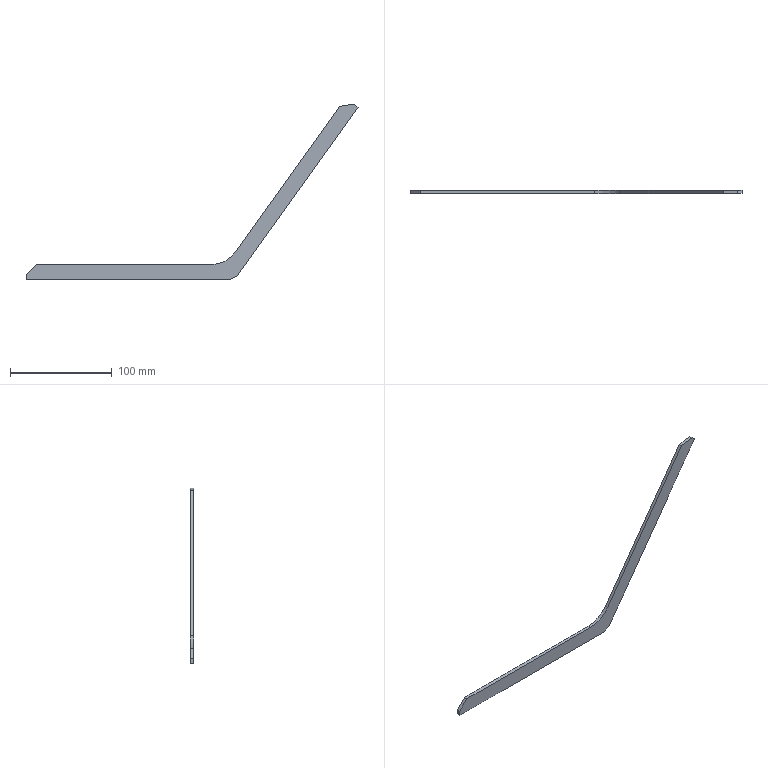Part | SolidWorks | features FlatPattern 1, SMBaseFlange 1, SheetMetal 1 | 1 solid | 12 faces | box 326.5 x 3.2 x 172.806 mm | volume 19256 mm3 | plane 11 | cylinder 1 | commonest cylinder face diameters 60 x1
STEP:
#1=CARTESIAN_POINT('',(0.,0.,0.));
#2=VERTEX_POINT('',#1);
#3=CARTESIAN_POINT('',(0.,0.,5.));
#4=VERTEX_POINT('',#3);
#5=CARTESIAN_POINT('',(0.,0.,0.));
#6=DIRECTION('',(0.,0.,1.));
#7=VECTOR('',#6,1000.);
#8=LINE('',#5,#7);
#9=EDGE_CURVE('',#2,#4,#8,.T.);
#10=ORIENTED_EDGE('',*,*,#9,.F.);
#11=CARTESIAN_POINT('',(0.,-3.2,0.));
#12=VERTEX_POINT('',#11);
#13=CARTESIAN_POINT('',(0.,-3.2,0.));
#14=DIRECTION('',(0.,1.,0.));
#15=VECTOR('',#14,1000.);
#16=LINE('',#13,#15);
#17=EDGE_CURVE('',#12,#2,#16,.T.);
#18=ORIENTED_EDGE('',*,*,#17,.F.);
#19=CARTESIAN_POINT('',(0.,-3.2,5.));
#20=VERTEX_POINT('',#19);
#21=CARTESIAN_POINT('',(0.,-3.2,0.));
#22=DIRECTION('',(0.,0.,1.));
#23=VECTOR('',#22,1000.);
#24=LINE('',#21,#23);
#25=EDGE_CURVE('',#12,#20,#24,.T.);
#26=ORIENTED_EDGE('',*,*,#25,.T.);
#27=CARTESIAN_POINT('',(0.,-3.2,5.));
#28=DIRECTION('',(0.,1.,0.));
#29=VECTOR('',#28,1000.);
#30=LINE('',#27,#29);
#31=EDGE_CURVE('',#20,#4,#30,.T.);
#32=ORIENTED_EDGE('',*,*,#31,.T.);
#33=EDGE_LOOP('',(#10,#18,#26,#32));
#34=FACE_OUTER_BOUND('',#33,.T.);
#35=CARTESIAN_POINT('',(0.,-3.2,0.));
#36=DIRECTION('',(-1.,0.,0.));
#37=DIRECTION('',(0.,0.,1.));
#38=AXIS2_PLACEMENT_3D('',#35,#36,#37);
#39=PLANE('',#38);
#40=ADVANCED_FACE('',(#34),#39,.T.);
#41=CARTESIAN_POINT('',(200.,0.,0.));
#42=VERTEX_POINT('',#41);
#43=CARTESIAN_POINT('',(0.,0.,0.));
#44=DIRECTION('',(-1.,0.,0.));
#45=VECTOR('',#44,1000.);
#46=LINE('',#43,#45);
#47=EDGE_CURVE('',#42,#2,#46,.T.);
#48=ORIENTED_EDGE('',*,*,#47,.F.);
#49=CARTESIAN_POINT('',(200.,-3.2,0.));
#50=VERTEX_POINT('',#49);
#51=CARTESIAN_POINT('',(200.,-3.2,0.));
#52=DIRECTION('',(0.,1.,0.));
#53=VECTOR('',#52,1000.);
#54=LINE('',#51,#53);
#55=EDGE_CURVE('',#50,#42,#54,.T.);
#56=ORIENTED_EDGE('',*,*,#55,.F.);
#57=CARTESIAN_POINT('',(0.,-3.2,0.));
#58=DIRECTION('',(-1.,0.,0.));
#59=VECTOR('',#58,1000.);
#60=LINE('',#57,#59);
#61=EDGE_CURVE('',#50,#12,#60,.T.);
#62=ORIENTED_EDGE('',*,*,#61,.T.);
#63=ORIENTED_EDGE('',*,*,#17,.T.);
#64=EDGE_LOOP('',(#48,#56,#62,#63));
#65=FACE_OUTER_BOUND('',#64,.T.);
#66=CARTESIAN_POINT('',(0.,-3.2,0.));
#67=DIRECTION('',(0.,0.,-1.));
#68=DIRECTION('',(-1.,0.,0.));
#69=AXIS2_PLACEMENT_3D('',#66,#67,#68);
#70=PLANE('',#69);
#71=ADVANCED_FACE('',(#65),#70,.T.);
#72=CARTESIAN_POINT('',(207.908,0.,4.067));
#73=VERTEX_POINT('',#72);
#74=CARTESIAN_POINT('',(200.,0.,0.));
#75=DIRECTION('',(-0.8893,0.,-0.4573));
#76=VECTOR('',#75,1000.);
#77=LINE('',#74,#76);
#78=EDGE_CURVE('',#73,#42,#77,.T.);
#79=ORIENTED_EDGE('',*,*,#78,.F.);
#80=CARTESIAN_POINT('',(207.908,-3.2,4.067));
#81=VERTEX_POINT('',#80);
#82=CARTESIAN_POINT('',(207.908,-3.2,4.067));
#83=DIRECTION('',(0.,1.,0.));
#84=VECTOR('',#83,1000.);
#85=LINE('',#82,#84);
#86=EDGE_CURVE('',#81,#73,#85,.T.);
#87=ORIENTED_EDGE('',*,*,#86,.F.);
#88=CARTESIAN_POINT('',(200.,-3.2,0.));
#89=DIRECTION('',(-0.8893,0.,-0.4573));
#90=VECTOR('',#89,1000.);
#91=LINE('',#88,#90);
#92=EDGE_CURVE('',#81,#50,#91,.T.);
#93=ORIENTED_EDGE('',*,*,#92,.T.);
#94=ORIENTED_EDGE('',*,*,#55,.T.);
#95=EDGE_LOOP('',(#79,#87,#93,#94));
#96=FACE_OUTER_BOUND('',#95,.T.);
#97=CARTESIAN_POINT('',(200.,-3.2,0.));
#98=DIRECTION('',(0.4573,0.,-0.8893));
#99=DIRECTION('',(-0.8893,0.,-0.4573));
#100=AXIS2_PLACEMENT_3D('',#97,#98,#99);
#101=PLANE('',#100);
#102=ADVANCED_FACE('',(#96),#101,.T.);
#103=CARTESIAN_POINT('',(326.5,0.,169.897));
#104=VERTEX_POINT('',#103);
#105=CARTESIAN_POINT('',(207.908,0.,4.067));
#106=DIRECTION('',(-0.5817,0.,-0.8134));
#107=VECTOR('',#106,1000.);
#108=LINE('',#105,#107);
#109=EDGE_CURVE('',#104,#73,#108,.T.);
#110=ORIENTED_EDGE('',*,*,#109,.F.);
#111=CARTESIAN_POINT('',(326.5,-3.2,169.897));
#112=VERTEX_POINT('',#111);
#113=CARTESIAN_POINT('',(326.5,-3.2,169.897));
#114=DIRECTION('',(0.,1.,0.));
#115=VECTOR('',#114,1000.);
#116=LINE('',#113,#115);
#117=EDGE_CURVE('',#112,#104,#116,.T.);
#118=ORIENTED_EDGE('',*,*,#117,.F.);
#119=CARTESIAN_POINT('',(207.908,-3.2,4.067));
#120=DIRECTION('',(-0.5817,0.,-0.8134));
#121=VECTOR('',#120,1000.);
#122=LINE('',#119,#121);
#123=EDGE_CURVE('',#112,#81,#122,.T.);
#124=ORIENTED_EDGE('',*,*,#123,.T.);
#125=ORIENTED_EDGE('',*,*,#86,.T.);
#126=EDGE_LOOP('',(#110,#118,#124,#125));
#127=FACE_OUTER_BOUND('',#126,.T.);
#128=CARTESIAN_POINT('',(207.908,-3.2,4.067));
#129=DIRECTION('',(0.8134,0.,-0.5817));
#130=DIRECTION('',(-0.5817,0.,-0.8134));
#131=AXIS2_PLACEMENT_3D('',#128,#129,#130);
#132=PLANE('',#131);
#133=ADVANCED_FACE('',(#127),#132,.T.);
#134=CARTESIAN_POINT('',(322.433,0.,172.806));
#135=VERTEX_POINT('',#134);
#136=CARTESIAN_POINT('',(322.433,0.,172.806));
#137=DIRECTION('',(0.8134,0.,-0.5817));
#138=VECTOR('',#137,1000.);
#139=LINE('',#136,#138);
#140=EDGE_CURVE('',#135,#104,#139,.T.);
#141=ORIENTED_EDGE('',*,*,#140,.F.);
#142=CARTESIAN_POINT('',(322.433,-3.2,172.806));
#143=VERTEX_POINT('',#142);
#144=CARTESIAN_POINT('',(322.433,-3.2,172.806));
#145=DIRECTION('',(0.,1.,0.));
#146=VECTOR('',#145,1000.);
#147=LINE('',#144,#146);
#148=EDGE_CURVE('',#143,#135,#147,.T.);
#149=ORIENTED_EDGE('',*,*,#148,.F.);
#150=CARTESIAN_POINT('',(322.433,-3.2,172.806));
#151=DIRECTION('',(0.8134,0.,-0.5817));
#152=VECTOR('',#151,1000.);
#153=LINE('',#150,#152);
#154=EDGE_CURVE('',#143,#112,#153,.T.);
#155=ORIENTED_EDGE('',*,*,#154,.T.);
#156=ORIENTED_EDGE('',*,*,#117,.T.);
#157=EDGE_LOOP('',(#141,#149,#155,#156));
#158=FACE_OUTER_BOUND('',#157,.T.);
#159=CARTESIAN_POINT('',(322.433,-3.2,172.806));
#160=DIRECTION('',(0.5817,0.,0.8134));
#161=DIRECTION('',(0.8134,0.,-0.5817));
#162=AXIS2_PLACEMENT_3D('',#159,#160,#161);
#163=PLANE('',#162);
#164=ADVANCED_FACE('',(#158),#163,.T.);
#165=CARTESIAN_POINT('',(308.482,0.,170.489));
#166=VERTEX_POINT('',#165);
#167=CARTESIAN_POINT('',(308.482,0.,170.489));
#168=DIRECTION('',(0.9865,0.,0.1638));
#169=VECTOR('',#168,1000.);
#170=LINE('',#167,#169);
#171=EDGE_CURVE('',#166,#135,#170,.T.);
#172=ORIENTED_EDGE('',*,*,#171,.F.);
#173=CARTESIAN_POINT('',(308.482,-3.2,170.489));
#174=VERTEX_POINT('',#173);
#175=CARTESIAN_POINT('',(308.482,-3.2,170.489));
#176=DIRECTION('',(0.,1.,0.));
#177=VECTOR('',#176,1000.);
#178=LINE('',#175,#177);
#179=EDGE_CURVE('',#174,#166,#178,.T.);
#180=ORIENTED_EDGE('',*,*,#179,.F.);
#181=CARTESIAN_POINT('',(308.482,-3.2,170.489));
#182=DIRECTION('',(0.9865,0.,0.1638));
#183=VECTOR('',#182,1000.);
#184=LINE('',#181,#183);
#185=EDGE_CURVE('',#174,#143,#184,.T.);
#186=ORIENTED_EDGE('',*,*,#185,.T.);
#187=ORIENTED_EDGE('',*,*,#148,.T.);
#188=EDGE_LOOP('',(#172,#180,#186,#187));
#189=FACE_OUTER_BOUND('',#188,.T.);
#190=CARTESIAN_POINT('',(308.482,-3.2,170.489));
#191=DIRECTION('',(-0.1638,0.,0.9865));
#192=DIRECTION('',(0.9865,0.,0.1638));
#193=AXIS2_PLACEMENT_3D('',#190,#191,#192);
#194=PLANE('',#193);
#195=ADVANCED_FACE('',(#189),#194,.T.);
#196=CARTESIAN_POINT('',(206.26,0.,27.549));
#197=VERTEX_POINT('',#196);
#198=CARTESIAN_POINT('',(206.26,0.,27.549));
#199=DIRECTION('',(0.5817,0.,0.8134));
#200=VECTOR('',#199,1000.);
#201=LINE('',#198,#200);
#202=EDGE_CURVE('',#197,#166,#201,.T.);
#203=ORIENTED_EDGE('',*,*,#202,.F.);
#204=CARTESIAN_POINT('',(206.26,-3.2,27.549));
#205=VERTEX_POINT('',#204);
#206=CARTESIAN_POINT('',(206.26,-3.2,27.549));
#207=DIRECTION('',(0.,1.,0.));
#208=VECTOR('',#207,1000.);
#209=LINE('',#206,#208);
#210=EDGE_CURVE('',#205,#197,#209,.T.);
#211=ORIENTED_EDGE('',*,*,#210,.F.);
#212=CARTESIAN_POINT('',(206.26,-3.2,27.549));
#213=DIRECTION('',(0.5817,0.,0.8134));
#214=VECTOR('',#213,1000.);
#215=LINE('',#212,#214);
#216=EDGE_CURVE('',#205,#174,#215,.T.);
#217=ORIENTED_EDGE('',*,*,#216,.T.);
#218=ORIENTED_EDGE('',*,*,#179,.T.);
#219=EDGE_LOOP('',(#203,#211,#217,#218));
#220=FACE_OUTER_BOUND('',#219,.T.);
#221=CARTESIAN_POINT('',(206.26,-3.2,27.549));
#222=DIRECTION('',(-0.8134,0.,0.5817));
#223=DIRECTION('',(0.5817,0.,0.8134));
#224=AXIS2_PLACEMENT_3D('',#221,#222,#223);
#225=PLANE('',#224);
#226=ADVANCED_FACE('',(#220),#225,.T.);
#227=CARTESIAN_POINT('',(181.858,0.,15.));
#228=VERTEX_POINT('',#227);
#229=CARTESIAN_POINT('',(181.858,0.,45.));
#230=DIRECTION('',(0.,-1.,0.));
#231=DIRECTION('',(0.,0.,-1.));
#232=AXIS2_PLACEMENT_3D('',#229,#230,#231);
#233=CIRCLE('',#232,30.);
#234=EDGE_CURVE('',#228,#197,#233,.T.);
#235=ORIENTED_EDGE('',*,*,#234,.F.);
#236=CARTESIAN_POINT('',(181.858,-3.2,15.));
#237=VERTEX_POINT('',#236);
#238=CARTESIAN_POINT('',(181.858,-3.2,15.));
#239=DIRECTION('',(0.,1.,0.));
#240=VECTOR('',#239,1000.);
#241=LINE('',#238,#240);
#242=EDGE_CURVE('',#237,#228,#241,.T.);
#243=ORIENTED_EDGE('',*,*,#242,.F.);
#244=CARTESIAN_POINT('',(181.858,-3.2,45.));
#245=DIRECTION('',(0.,-1.,0.));
#246=DIRECTION('',(0.,0.,-1.));
#247=AXIS2_PLACEMENT_3D('',#244,#245,#246);
#248=CIRCLE('',#247,30.);
#249=EDGE_CURVE('',#237,#205,#248,.T.);
#250=ORIENTED_EDGE('',*,*,#249,.T.);
#251=ORIENTED_EDGE('',*,*,#210,.T.);
#252=EDGE_LOOP('',(#235,#243,#250,#251));
#253=FACE_OUTER_BOUND('',#252,.T.);
#254=CARTESIAN_POINT('',(181.858,-3.2,45.));
#255=DIRECTION('',(0.,1.,0.));
#256=DIRECTION('',(0.,0.,1.));
#257=AXIS2_PLACEMENT_3D('',#254,#255,#256);
#258=CYLINDRICAL_SURFACE('',#257,30.);
#259=ADVANCED_FACE('',(#253),#258,.F.);
#260=CARTESIAN_POINT('',(10.,0.,15.));
#261=VERTEX_POINT('',#260);
#262=CARTESIAN_POINT('',(10.,0.,15.));
#263=DIRECTION('',(1.,0.,0.));
#264=VECTOR('',#263,1000.);
#265=LINE('',#262,#264);
#266=EDGE_CURVE('',#261,#228,#265,.T.);
#267=ORIENTED_EDGE('',*,*,#266,.F.);
#268=CARTESIAN_POINT('',(10.,-3.2,15.));
#269=VERTEX_POINT('',#268);
#270=CARTESIAN_POINT('',(10.,-3.2,15.));
#271=DIRECTION('',(0.,1.,0.));
#272=VECTOR('',#271,1000.);
#273=LINE('',#270,#272);
#274=EDGE_CURVE('',#269,#261,#273,.T.);
#275=ORIENTED_EDGE('',*,*,#274,.F.);
#276=CARTESIAN_POINT('',(10.,-3.2,15.));
#277=DIRECTION('',(1.,0.,0.));
#278=VECTOR('',#277,1000.);
#279=LINE('',#276,#278);
#280=EDGE_CURVE('',#269,#237,#279,.T.);
#281=ORIENTED_EDGE('',*,*,#280,.T.);
#282=ORIENTED_EDGE('',*,*,#242,.T.);
#283=EDGE_LOOP('',(#267,#275,#281,#282));
#284=FACE_OUTER_BOUND('',#283,.T.);
#285=CARTESIAN_POINT('',(10.,-3.2,15.));
#286=DIRECTION('',(0.,0.,1.));
#287=DIRECTION('',(1.,0.,0.));
#288=AXIS2_PLACEMENT_3D('',#285,#286,#287);
#289=PLANE('',#288);
#290=ADVANCED_FACE('',(#284),#289,.T.);
#291=CARTESIAN_POINT('',(0.,0.,5.));
#292=DIRECTION('',(0.7071,0.,0.7071));
#293=VECTOR('',#292,1000.);
#294=LINE('',#291,#293);
#295=EDGE_CURVE('',#4,#261,#294,.T.);
#296=ORIENTED_EDGE('',*,*,#295,.F.);
#297=ORIENTED_EDGE('',*,*,#31,.F.);
#298=CARTESIAN_POINT('',(0.,-3.2,5.));
#299=DIRECTION('',(0.7071,0.,0.7071));
#300=VECTOR('',#299,1000.);
#301=LINE('',#298,#300);
#302=EDGE_CURVE('',#20,#269,#301,.T.);
#303=ORIENTED_EDGE('',*,*,#302,.T.);
#304=ORIENTED_EDGE('',*,*,#274,.T.);
#305=EDGE_LOOP('',(#296,#297,#303,#304));
#306=FACE_OUTER_BOUND('',#305,.T.);
#307=CARTESIAN_POINT('',(0.,-3.2,5.));
#308=DIRECTION('',(-0.7071,0.,0.7071));
#309=DIRECTION('',(0.7071,0.,0.7071));
#310=AXIS2_PLACEMENT_3D('',#307,#308,#309);
#311=PLANE('',#310);
#312=ADVANCED_FACE('',(#306),#311,.T.);
#313=ORIENTED_EDGE('',*,*,#25,.F.);
#314=ORIENTED_EDGE('',*,*,#61,.F.);
#315=ORIENTED_EDGE('',*,*,#92,.F.);
#316=ORIENTED_EDGE('',*,*,#123,.F.);
#317=ORIENTED_EDGE('',*,*,#154,.F.);
#318=ORIENTED_EDGE('',*,*,#185,.F.);
#319=ORIENTED_EDGE('',*,*,#216,.F.);
#320=ORIENTED_EDGE('',*,*,#249,.F.);
#321=ORIENTED_EDGE('',*,*,#280,.F.);
#322=ORIENTED_EDGE('',*,*,#302,.F.);
#323=EDGE_LOOP('',(#313,#314,#315,#316,#317,#318,#319,#320,#321,#322));
#324=FACE_OUTER_BOUND('',#323,.T.);
#325=CARTESIAN_POINT('',(181.858,-3.2,45.));
#326=DIRECTION('',(0.,-1.,0.));
#327=DIRECTION('',(0.,0.,-1.));
#328=AXIS2_PLACEMENT_3D('',#325,#326,#327);
#329=PLANE('',#328);
#330=ADVANCED_FACE('',(#324),#329,.T.);
#331=ORIENTED_EDGE('',*,*,#9,.T.);
#332=ORIENTED_EDGE('',*,*,#295,.T.);
#333=ORIENTED_EDGE('',*,*,#266,.T.);
#334=ORIENTED_EDGE('',*,*,#234,.T.);
#335=ORIENTED_EDGE('',*,*,#202,.T.);
#336=ORIENTED_EDGE('',*,*,#171,.T.);
#337=ORIENTED_EDGE('',*,*,#140,.T.);
#338=ORIENTED_EDGE('',*,*,#109,.T.);
#339=ORIENTED_EDGE('',*,*,#78,.T.);
#340=ORIENTED_EDGE('',*,*,#47,.T.);
#341=EDGE_LOOP('',(#331,#332,#333,#334,#335,#336,#337,#338,#339,#340));
#342=FACE_OUTER_BOUND('',#341,.T.);
#343=CARTESIAN_POINT('',(181.858,0.,45.));
#344=DIRECTION('',(0.,-1.,0.));
#345=DIRECTION('',(0.,0.,-1.));
#346=AXIS2_PLACEMENT_3D('',#343,#344,#345);
#347=PLANE('',#346);
#348=ADVANCED_FACE('',(#342),#347,.F.);
#349=CLOSED_SHELL('',(#40,#71,#102,#133,#164,#195,#226,#259,#290,#312,#330,#348));
#350=MANIFOLD_SOLID_BREP('',#349);
#351=CARTESIAN_POINT('',(0.,0.,0.));
#352=DIRECTION('',(0.,0.,1.));
#353=DIRECTION('',(1.,0.,0.));
#354=AXIS2_PLACEMENT_3D('',#351,#352,#353);
#355=(LENGTH_UNIT()NAMED_UNIT(*)SI_UNIT(.MILLI.,.METRE.));
#356=UNCERTAINTY_MEASURE_WITH_UNIT(LENGTH_MEASURE(0.00001),#355,'','');
#357=(NAMED_UNIT(*)PLANE_ANGLE_UNIT()SI_UNIT($,.RADIAN.));
#358=(NAMED_UNIT(*)SI_UNIT($,.STERADIAN.)SOLID_ANGLE_UNIT());
#359=(GEOMETRIC_REPRESENTATION_CONTEXT(3)GLOBAL_UNCERTAINTY_ASSIGNED_CONTEXT((#356))GLOBAL_UNIT_ASSIGNED_CONTEXT((#355,#357,#358))REPRESENTATION_CONTEXT('',''));
#360=ADVANCED_BREP_SHAPE_REPRESENTATION('',(#350,#354),#359);